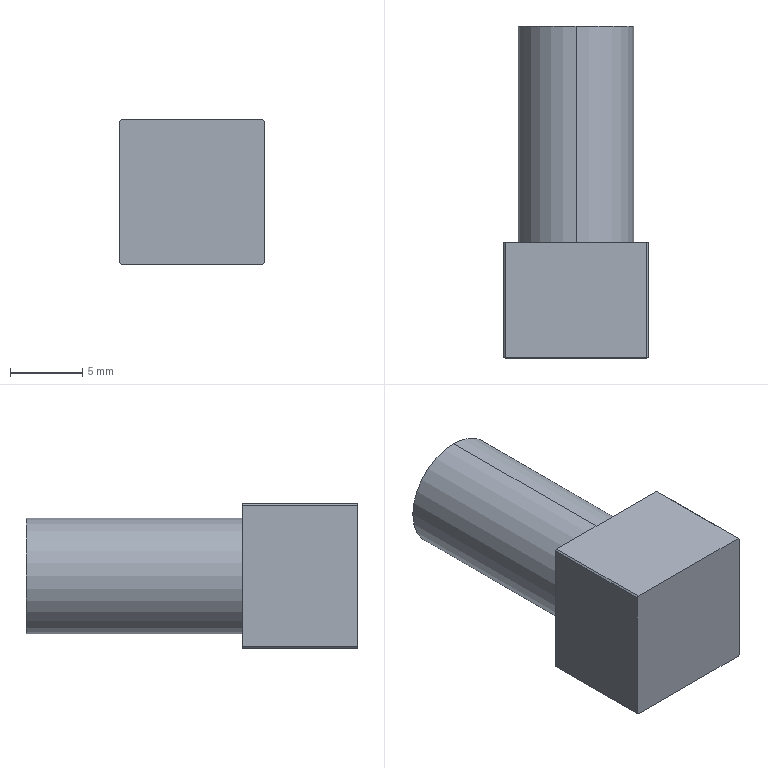Part | STEP file | 1 solid | 13 faces | box 10 x 23 x 10 mm | volume 1554 mm3 | plane 7 | cylinder 6 | commonest cylinder face diameters 14 x4 8 x2
STEP:
#1=CARTESIAN_POINT('',(0.,0.,0.));
#2=DIRECTION('',(0.,0.,1.));
#3=DIRECTION('',(1.,0.,0.));
#4=AXIS2_PLACEMENT_3D('',#1,#2,#3);
#5=CARTESIAN_POINT('',(0.,23.,-4.));
#6=VERTEX_POINT('',#5);
#7=CARTESIAN_POINT('',(0.,23.,4.));
#8=VERTEX_POINT('',#7);
#9=CARTESIAN_POINT('',(0.,23.,0.));
#10=DIRECTION('',(0.,-1.,0.));
#11=DIRECTION('',(0.,0.,-1.));
#12=AXIS2_PLACEMENT_3D('',#9,#10,#11);
#13=CIRCLE('',#12,4.);
#14=CARTESIAN_POINT('',(0.,0.,0.));
#15=DIRECTION('',(0.,-1.,0.));
#16=DIRECTION('',(0.,0.,-1.));
#17=AXIS2_PLACEMENT_3D('',#14,#15,#16);
#18=CYLINDRICAL_SURFACE('',#17,4.);
#19=CARTESIAN_POINT('',(0.,-23.));
#20=DIRECTION('',(1.,0.));
#21=VECTOR('',#20,1.);
#22=LINE('',#19,#21);
#23=(GEOMETRIC_REPRESENTATION_CONTEXT(2)PARAMETRIC_REPRESENTATION_CONTEXT()REPRESENTATION_CONTEXT('',''));
#24=DEFINITIONAL_REPRESENTATION('',(#22),#23);
#25=PCURVE('',#18,#24);
#26=CARTESIAN_POINT('',(4.,23.,0.));
#27=DIRECTION('',(0.,1.,0.));
#28=DIRECTION('',(0.,0.,1.));
#29=AXIS2_PLACEMENT_3D('',#26,#27,#28);
#30=PLANE('',#29);
#31=CARTESIAN_POINT('',(-4.,-4.));
#32=CARTESIAN_POINT('',(-4.,2.928));
#33=CARTESIAN_POINT('',(2.,-0.5359));
#34=CARTESIAN_POINT('',(8.,-4.));
#35=CARTESIAN_POINT('',(2.,-7.464));
#36=CARTESIAN_POINT('',(-4.,-10.928));
#37=CARTESIAN_POINT('',(-4.,-4.));
#38=(BOUNDED_CURVE()B_SPLINE_CURVE(2,(#31,#32,#33,#34,#35,#36,#37),.UNSPECIFIED.,.T.,.F.)B_SPLINE_CURVE_WITH_KNOTS((1,2,2,2,2,1),(-2.094,0.,2.094,4.189,6.283,8.378),.UNSPECIFIED.)CURVE()GEOMETRIC_REPRESENTATION_ITEM()RATIONAL_B_SPLINE_CURVE((1.,0.5,1.,0.5,1.,0.5,1.))REPRESENTATION_ITEM(''));
#39=(GEOMETRIC_REPRESENTATION_CONTEXT(2)PARAMETRIC_REPRESENTATION_CONTEXT()REPRESENTATION_CONTEXT('',''));
#40=DEFINITIONAL_REPRESENTATION('',(#38),#39);
#41=PCURVE('',#30,#40);
#42=SURFACE_CURVE('',#13,(#25,#41),.PCURVE_S1.);
#43=EDGE_CURVE('',#6,#8,#42,.T.);
#44=ORIENTED_EDGE('',*,*,#43,.T.);
#45=CARTESIAN_POINT('',(0.,8.,4.));
#46=VERTEX_POINT('',#45);
#47=CARTESIAN_POINT('',(0.,0.,4.));
#48=DIRECTION('',(0.,-1.,0.));
#49=VECTOR('',#48,1.);
#50=LINE('',#47,#49);
#51=CARTESIAN_POINT('',(3.142,0.));
#52=DIRECTION('',(0.,1.));
#53=VECTOR('',#52,1.);
#54=LINE('',#51,#53);
#55=(GEOMETRIC_REPRESENTATION_CONTEXT(2)PARAMETRIC_REPRESENTATION_CONTEXT()REPRESENTATION_CONTEXT('',''));
#56=DEFINITIONAL_REPRESENTATION('',(#54),#55);
#57=PCURVE('',#18,#56);
#58=CARTESIAN_POINT('',(0.,0.,0.));
#59=DIRECTION('',(0.,-1.,0.));
#60=DIRECTION('',(0.,0.,-1.));
#61=AXIS2_PLACEMENT_3D('',#58,#59,#60);
#62=CYLINDRICAL_SURFACE('',#61,4.);
#63=CARTESIAN_POINT('',(3.142,0.));
#64=DIRECTION('',(0.,1.));
#65=VECTOR('',#64,1.);
#66=LINE('',#63,#65);
#67=(GEOMETRIC_REPRESENTATION_CONTEXT(2)PARAMETRIC_REPRESENTATION_CONTEXT()REPRESENTATION_CONTEXT('',''));
#68=DEFINITIONAL_REPRESENTATION('',(#66),#67);
#69=PCURVE('',#62,#68);
#70=SURFACE_CURVE('',#50,(#57,#69),.PCURVE_S1.);
#71=EDGE_CURVE('',#8,#46,#70,.T.);
#72=ORIENTED_EDGE('',*,*,#71,.T.);
#73=CARTESIAN_POINT('',(0.,8.,-4.));
#74=VERTEX_POINT('',#73);
#75=CARTESIAN_POINT('',(0.,8.,0.));
#76=DIRECTION('',(0.,-1.,0.));
#77=DIRECTION('',(0.,0.,-1.));
#78=AXIS2_PLACEMENT_3D('',#75,#76,#77);
#79=CIRCLE('',#78,4.);
#80=CARTESIAN_POINT('',(0.,-8.));
#81=DIRECTION('',(1.,0.));
#82=VECTOR('',#81,1.);
#83=LINE('',#80,#82);
#84=(GEOMETRIC_REPRESENTATION_CONTEXT(2)PARAMETRIC_REPRESENTATION_CONTEXT()REPRESENTATION_CONTEXT('',''));
#85=DEFINITIONAL_REPRESENTATION('',(#83),#84);
#86=PCURVE('',#18,#85);
#87=CARTESIAN_POINT('',(7.,8.,0.));
#88=DIRECTION('',(0.,1.,0.));
#89=DIRECTION('',(0.,0.,1.));
#90=AXIS2_PLACEMENT_3D('',#87,#88,#89);
#91=PLANE('',#90);
#92=CARTESIAN_POINT('',(-4.,-7.));
#93=CARTESIAN_POINT('',(-4.,-0.0718));
#94=CARTESIAN_POINT('',(2.,-3.536));
#95=CARTESIAN_POINT('',(8.,-7.));
#96=CARTESIAN_POINT('',(2.,-10.464));
#97=CARTESIAN_POINT('',(-4.,-13.928));
#98=CARTESIAN_POINT('',(-4.,-7.));
#99=(BOUNDED_CURVE()B_SPLINE_CURVE(2,(#92,#93,#94,#95,#96,#97,#98),.UNSPECIFIED.,.T.,.F.)B_SPLINE_CURVE_WITH_KNOTS((1,2,2,2,2,1),(-2.094,0.,2.094,4.189,6.283,8.378),.UNSPECIFIED.)CURVE()GEOMETRIC_REPRESENTATION_ITEM()RATIONAL_B_SPLINE_CURVE((1.,0.5,1.,0.5,1.,0.5,1.))REPRESENTATION_ITEM(''));
#100=(GEOMETRIC_REPRESENTATION_CONTEXT(2)PARAMETRIC_REPRESENTATION_CONTEXT()REPRESENTATION_CONTEXT('',''));
#101=DEFINITIONAL_REPRESENTATION('',(#99),#100);
#102=PCURVE('',#91,#101);
#103=SURFACE_CURVE('',#79,(#86,#102),.PCURVE_S1.);
#104=EDGE_CURVE('',#74,#46,#103,.T.);
#105=ORIENTED_EDGE('',*,*,#104,.F.);
#106=CARTESIAN_POINT('',(0.,0.,-4.));
#107=DIRECTION('',(0.,-1.,0.));
#108=VECTOR('',#107,1.);
#109=LINE('',#106,#108);
#110=CARTESIAN_POINT('',(0.,0.));
#111=DIRECTION('',(0.,1.));
#112=VECTOR('',#111,1.);
#113=LINE('',#110,#112);
#114=(GEOMETRIC_REPRESENTATION_CONTEXT(2)PARAMETRIC_REPRESENTATION_CONTEXT()REPRESENTATION_CONTEXT('',''));
#115=DEFINITIONAL_REPRESENTATION('',(#113),#114);
#116=PCURVE('',#18,#115);
#117=CARTESIAN_POINT('',(6.283,0.));
#118=DIRECTION('',(0.,1.));
#119=VECTOR('',#118,1.);
#120=LINE('',#117,#119);
#121=(GEOMETRIC_REPRESENTATION_CONTEXT(2)PARAMETRIC_REPRESENTATION_CONTEXT()REPRESENTATION_CONTEXT('',''));
#122=DEFINITIONAL_REPRESENTATION('',(#120),#121);
#123=PCURVE('',#62,#122);
#124=SURFACE_CURVE('',#109,(#116,#123),.PCURVE_S1.);
#125=EDGE_CURVE('',#6,#74,#124,.T.);
#126=ORIENTED_EDGE('',*,*,#125,.F.);
#127=EDGE_LOOP('',(#44,#72,#105,#126));
#128=FACE_BOUND('',#127,.T.);
#129=ADVANCED_FACE('',(#128),#18,.T.);
#130=CARTESIAN_POINT('',(5.,0.,-4.899));
#131=VERTEX_POINT('',#130);
#132=CARTESIAN_POINT('',(5.,8.,-4.899));
#133=VERTEX_POINT('',#132);
#134=CARTESIAN_POINT('',(5.,0.,-4.899));
#135=DIRECTION('',(0.,1.,0.));
#136=VECTOR('',#135,1.);
#137=LINE('',#134,#136);
#138=CARTESIAN_POINT('',(0.,0.,0.));
#139=DIRECTION('',(0.,-1.,0.));
#140=DIRECTION('',(0.,0.,-1.));
#141=AXIS2_PLACEMENT_3D('',#138,#139,#140);
#142=CYLINDRICAL_SURFACE('',#141,7.);
#143=CARTESIAN_POINT('',(0.7956,0.));
#144=DIRECTION('',(0.,-1.));
#145=VECTOR('',#144,1.);
#146=LINE('',#143,#145);
#147=(GEOMETRIC_REPRESENTATION_CONTEXT(2)PARAMETRIC_REPRESENTATION_CONTEXT()REPRESENTATION_CONTEXT('',''));
#148=DEFINITIONAL_REPRESENTATION('',(#146),#147);
#149=PCURVE('',#142,#148);
#150=CARTESIAN_POINT('',(5.,23.,8.094));
#151=DIRECTION('',(-1.,0.,0.));
#152=DIRECTION('',(0.,0.,1.));
#153=AXIS2_PLACEMENT_3D('',#150,#151,#152);
#154=PLANE('',#153);
#155=CARTESIAN_POINT('',(-12.993,-23.));
#156=DIRECTION('',(0.,1.));
#157=VECTOR('',#156,1.);
#158=LINE('',#155,#157);
#159=(GEOMETRIC_REPRESENTATION_CONTEXT(2)PARAMETRIC_REPRESENTATION_CONTEXT()REPRESENTATION_CONTEXT('',''));
#160=DEFINITIONAL_REPRESENTATION('',(#158),#159);
#161=PCURVE('',#154,#160);
#162=SURFACE_CURVE('',#137,(#149,#161),.PCURVE_S1.);
#163=EDGE_CURVE('',#131,#133,#162,.T.);
#164=ORIENTED_EDGE('',*,*,#163,.F.);
#165=CARTESIAN_POINT('',(4.899,0.,-5.));
#166=VERTEX_POINT('',#165);
#167=CARTESIAN_POINT('',(0.,0.,0.));
#168=DIRECTION('',(0.,-1.,0.));
#169=DIRECTION('',(0.,0.,-1.));
#170=AXIS2_PLACEMENT_3D('',#167,#168,#169);
#171=CIRCLE('',#170,7.);
#172=CARTESIAN_POINT('',(0.,0.));
#173=DIRECTION('',(1.,0.));
#174=VECTOR('',#173,1.);
#175=LINE('',#172,#174);
#176=(GEOMETRIC_REPRESENTATION_CONTEXT(2)PARAMETRIC_REPRESENTATION_CONTEXT()REPRESENTATION_CONTEXT('',''));
#177=DEFINITIONAL_REPRESENTATION('',(#175),#176);
#178=PCURVE('',#142,#177);
#179=CARTESIAN_POINT('',(0.,0.,0.));
#180=DIRECTION('',(0.,-1.,0.));
#181=DIRECTION('',(0.,0.,-1.));
#182=AXIS2_PLACEMENT_3D('',#179,#180,#181);
#183=PLANE('',#182);
#184=CARTESIAN_POINT('',(0.,0.));
#185=DIRECTION('',(1.,0.));
#186=AXIS2_PLACEMENT_2D('',#184,#185);
#187=CIRCLE('',#186,7.);
#188=(GEOMETRIC_REPRESENTATION_CONTEXT(2)PARAMETRIC_REPRESENTATION_CONTEXT()REPRESENTATION_CONTEXT('',''));
#189=DEFINITIONAL_REPRESENTATION('',(#187),#188);
#190=PCURVE('',#183,#189);
#191=SURFACE_CURVE('',#171,(#178,#190),.PCURVE_S1.);
#192=EDGE_CURVE('',#166,#131,#191,.T.);
#193=ORIENTED_EDGE('',*,*,#192,.F.);
#194=CARTESIAN_POINT('',(4.899,8.,-5.));
#195=VERTEX_POINT('',#194);
#196=CARTESIAN_POINT('',(4.899,0.,-5.));
#197=DIRECTION('',(0.,-1.,0.));
#198=VECTOR('',#197,1.);
#199=LINE('',#196,#198);
#200=CARTESIAN_POINT('',(0.7752,0.));
#201=DIRECTION('',(0.,1.));
#202=VECTOR('',#201,1.);
#203=LINE('',#200,#202);
#204=(GEOMETRIC_REPRESENTATION_CONTEXT(2)PARAMETRIC_REPRESENTATION_CONTEXT()REPRESENTATION_CONTEXT('',''));
#205=DEFINITIONAL_REPRESENTATION('',(#203),#204);
#206=PCURVE('',#142,#205);
#207=CARTESIAN_POINT('',(-14.765,23.,-5.));
#208=DIRECTION('',(0.,0.,1.));
#209=DIRECTION('',(1.,0.,0.));
#210=AXIS2_PLACEMENT_3D('',#207,#208,#209);
#211=PLANE('',#210);
#212=CARTESIAN_POINT('',(19.664,-23.));
#213=DIRECTION('',(0.,-1.));
#214=VECTOR('',#213,1.);
#215=LINE('',#212,#214);
#216=(GEOMETRIC_REPRESENTATION_CONTEXT(2)PARAMETRIC_REPRESENTATION_CONTEXT()REPRESENTATION_CONTEXT('',''));
#217=DEFINITIONAL_REPRESENTATION('',(#215),#216);
#218=PCURVE('',#211,#217);
#219=SURFACE_CURVE('',#199,(#206,#218),.PCURVE_S1.);
#220=EDGE_CURVE('',#195,#166,#219,.T.);
#221=ORIENTED_EDGE('',*,*,#220,.F.);
#222=CARTESIAN_POINT('',(0.,8.,0.));
#223=DIRECTION('',(0.,-1.,0.));
#224=DIRECTION('',(0.,0.,-1.));
#225=AXIS2_PLACEMENT_3D('',#222,#223,#224);
#226=CIRCLE('',#225,7.);
#227=CARTESIAN_POINT('',(0.,-8.));
#228=DIRECTION('',(1.,0.));
#229=VECTOR('',#228,1.);
#230=LINE('',#227,#229);
#231=(GEOMETRIC_REPRESENTATION_CONTEXT(2)PARAMETRIC_REPRESENTATION_CONTEXT()REPRESENTATION_CONTEXT('',''));
#232=DEFINITIONAL_REPRESENTATION('',(#230),#231);
#233=PCURVE('',#142,#232);
#234=CARTESIAN_POINT('',(-7.,-7.));
#235=CARTESIAN_POINT('',(-7.,5.124));
#236=CARTESIAN_POINT('',(3.5,-0.9378));
#237=CARTESIAN_POINT('',(14.,-7.));
#238=CARTESIAN_POINT('',(3.5,-13.062));
#239=CARTESIAN_POINT('',(-7.,-19.124));
#240=CARTESIAN_POINT('',(-7.,-7.));
#241=(BOUNDED_CURVE()B_SPLINE_CURVE(2,(#234,#235,#236,#237,#238,#239,#240),.UNSPECIFIED.,.T.,.F.)B_SPLINE_CURVE_WITH_KNOTS((1,2,2,2,2,1),(-2.094,0.,2.094,4.189,6.283,8.378),.UNSPECIFIED.)CURVE()GEOMETRIC_REPRESENTATION_ITEM()RATIONAL_B_SPLINE_CURVE((1.,0.5,1.,0.5,1.,0.5,1.))REPRESENTATION_ITEM(''));
#242=(GEOMETRIC_REPRESENTATION_CONTEXT(2)PARAMETRIC_REPRESENTATION_CONTEXT()REPRESENTATION_CONTEXT('',''));
#243=DEFINITIONAL_REPRESENTATION('',(#241),#242);
#244=PCURVE('',#91,#243);
#245=SURFACE_CURVE('',#226,(#233,#244),.PCURVE_S1.);
#246=EDGE_CURVE('',#195,#133,#245,.T.);
#247=ORIENTED_EDGE('',*,*,#246,.T.);
#248=EDGE_LOOP('',(#164,#193,#221,#247));
#249=FACE_BOUND('',#248,.T.);
#250=ADVANCED_FACE('',(#249),#142,.T.);
#251=CARTESIAN_POINT('',(-5.,0.,4.899));
#252=VERTEX_POINT('',#251);
#253=CARTESIAN_POINT('',(-5.,8.,4.899));
#254=VERTEX_POINT('',#253);
#255=CARTESIAN_POINT('',(-5.,0.,4.899));
#256=DIRECTION('',(0.,1.,0.));
#257=VECTOR('',#256,1.);
#258=LINE('',#255,#257);
#259=CARTESIAN_POINT('',(0.,0.,0.));
#260=DIRECTION('',(0.,-1.,0.));
#261=DIRECTION('',(0.,0.,-1.));
#262=AXIS2_PLACEMENT_3D('',#259,#260,#261);
#263=CYLINDRICAL_SURFACE('',#262,7.);
#264=CARTESIAN_POINT('',(3.937,0.));
#265=DIRECTION('',(0.,-1.));
#266=VECTOR('',#265,1.);
#267=LINE('',#264,#266);
#268=(GEOMETRIC_REPRESENTATION_CONTEXT(2)PARAMETRIC_REPRESENTATION_CONTEXT()REPRESENTATION_CONTEXT('',''));
#269=DEFINITIONAL_REPRESENTATION('',(#267),#268);
#270=PCURVE('',#263,#269);
#271=CARTESIAN_POINT('',(-5.,23.,8.094));
#272=DIRECTION('',(1.,0.,0.));
#273=DIRECTION('',(0.,0.,-1.));
#274=AXIS2_PLACEMENT_3D('',#271,#272,#273);
#275=PLANE('',#274);
#276=CARTESIAN_POINT('',(3.195,-23.));
#277=DIRECTION('',(0.,1.));
#278=VECTOR('',#277,1.);
#279=LINE('',#276,#278);
#280=(GEOMETRIC_REPRESENTATION_CONTEXT(2)PARAMETRIC_REPRESENTATION_CONTEXT()REPRESENTATION_CONTEXT('',''));
#281=DEFINITIONAL_REPRESENTATION('',(#279),#280);
#282=PCURVE('',#275,#281);
#283=SURFACE_CURVE('',#258,(#270,#282),.PCURVE_S1.);
#284=EDGE_CURVE('',#252,#254,#283,.T.);
#285=ORIENTED_EDGE('',*,*,#284,.F.);
#286=CARTESIAN_POINT('',(-4.899,0.,5.));
#287=VERTEX_POINT('',#286);
#288=CARTESIAN_POINT('',(0.,0.,0.));
#289=DIRECTION('',(0.,-1.,0.));
#290=DIRECTION('',(0.,0.,-1.));
#291=AXIS2_PLACEMENT_3D('',#288,#289,#290);
#292=CIRCLE('',#291,7.);
#293=CARTESIAN_POINT('',(0.,0.));
#294=DIRECTION('',(1.,0.));
#295=VECTOR('',#294,1.);
#296=LINE('',#293,#295);
#297=(GEOMETRIC_REPRESENTATION_CONTEXT(2)PARAMETRIC_REPRESENTATION_CONTEXT()REPRESENTATION_CONTEXT('',''));
#298=DEFINITIONAL_REPRESENTATION('',(#296),#297);
#299=PCURVE('',#263,#298);
#300=CARTESIAN_POINT('',(0.,0.));
#301=DIRECTION('',(1.,0.));
#302=AXIS2_PLACEMENT_2D('',#300,#301);
#303=CIRCLE('',#302,7.);
#304=(GEOMETRIC_REPRESENTATION_CONTEXT(2)PARAMETRIC_REPRESENTATION_CONTEXT()REPRESENTATION_CONTEXT('',''));
#305=DEFINITIONAL_REPRESENTATION('',(#303),#304);
#306=PCURVE('',#183,#305);
#307=SURFACE_CURVE('',#292,(#299,#306),.PCURVE_S1.);
#308=EDGE_CURVE('',#287,#252,#307,.T.);
#309=ORIENTED_EDGE('',*,*,#308,.F.);
#310=CARTESIAN_POINT('',(-4.899,8.,5.));
#311=VERTEX_POINT('',#310);
#312=CARTESIAN_POINT('',(-4.899,0.,5.));
#313=DIRECTION('',(0.,-1.,0.));
#314=VECTOR('',#313,1.);
#315=LINE('',#312,#314);
#316=CARTESIAN_POINT('',(3.917,0.));
#317=DIRECTION('',(0.,1.));
#318=VECTOR('',#317,1.);
#319=LINE('',#316,#318);
#320=(GEOMETRIC_REPRESENTATION_CONTEXT(2)PARAMETRIC_REPRESENTATION_CONTEXT()REPRESENTATION_CONTEXT('',''));
#321=DEFINITIONAL_REPRESENTATION('',(#319),#320);
#322=PCURVE('',#263,#321);
#323=CARTESIAN_POINT('',(-11.017,23.,5.));
#324=DIRECTION('',(0.,0.,-1.));
#325=DIRECTION('',(-1.,0.,0.));
#326=AXIS2_PLACEMENT_3D('',#323,#324,#325);
#327=PLANE('',#326);
#328=CARTESIAN_POINT('',(-6.118,-23.));
#329=DIRECTION('',(0.,-1.));
#330=VECTOR('',#329,1.);
#331=LINE('',#328,#330);
#332=(GEOMETRIC_REPRESENTATION_CONTEXT(2)PARAMETRIC_REPRESENTATION_CONTEXT()REPRESENTATION_CONTEXT('',''));
#333=DEFINITIONAL_REPRESENTATION('',(#331),#332);
#334=PCURVE('',#327,#333);
#335=SURFACE_CURVE('',#315,(#322,#334),.PCURVE_S1.);
#336=EDGE_CURVE('',#311,#287,#335,.T.);
#337=ORIENTED_EDGE('',*,*,#336,.F.);
#338=CARTESIAN_POINT('',(0.,8.,0.));
#339=DIRECTION('',(0.,-1.,0.));
#340=DIRECTION('',(0.,0.,-1.));
#341=AXIS2_PLACEMENT_3D('',#338,#339,#340);
#342=CIRCLE('',#341,7.);
#343=CARTESIAN_POINT('',(0.,-8.));
#344=DIRECTION('',(1.,0.));
#345=VECTOR('',#344,1.);
#346=LINE('',#343,#345);
#347=(GEOMETRIC_REPRESENTATION_CONTEXT(2)PARAMETRIC_REPRESENTATION_CONTEXT()REPRESENTATION_CONTEXT('',''));
#348=DEFINITIONAL_REPRESENTATION('',(#346),#347);
#349=PCURVE('',#263,#348);
#350=CARTESIAN_POINT('',(-7.,-7.));
#351=CARTESIAN_POINT('',(-7.,5.124));
#352=CARTESIAN_POINT('',(3.5,-0.9378));
#353=CARTESIAN_POINT('',(14.,-7.));
#354=CARTESIAN_POINT('',(3.5,-13.062));
#355=CARTESIAN_POINT('',(-7.,-19.124));
#356=CARTESIAN_POINT('',(-7.,-7.));
#357=(BOUNDED_CURVE()B_SPLINE_CURVE(2,(#350,#351,#352,#353,#354,#355,#356),.UNSPECIFIED.,.T.,.F.)B_SPLINE_CURVE_WITH_KNOTS((1,2,2,2,2,1),(-2.094,0.,2.094,4.189,6.283,8.378),.UNSPECIFIED.)CURVE()GEOMETRIC_REPRESENTATION_ITEM()RATIONAL_B_SPLINE_CURVE((1.,0.5,1.,0.5,1.,0.5,1.))REPRESENTATION_ITEM(''));
#358=(GEOMETRIC_REPRESENTATION_CONTEXT(2)PARAMETRIC_REPRESENTATION_CONTEXT()REPRESENTATION_CONTEXT('',''));
#359=DEFINITIONAL_REPRESENTATION('',(#357),#358);
#360=PCURVE('',#91,#359);
#361=SURFACE_CURVE('',#342,(#349,#360),.PCURVE_S1.);
#362=EDGE_CURVE('',#311,#254,#361,.T.);
#363=ORIENTED_EDGE('',*,*,#362,.T.);
#364=EDGE_LOOP('',(#285,#309,#337,#363));
#365=FACE_BOUND('',#364,.T.);
#366=ADVANCED_FACE('',(#365),#263,.T.);
#367=CARTESIAN_POINT('',(5.,8.,4.899));
#368=VERTEX_POINT('',#367);
#369=CARTESIAN_POINT('',(5.,0.,4.899));
#370=VERTEX_POINT('',#369);
#371=CARTESIAN_POINT('',(5.,0.,4.899));
#372=DIRECTION('',(0.,-1.,0.));
#373=VECTOR('',#372,1.);
#374=LINE('',#371,#373);
#375=CARTESIAN_POINT('',(0.,0.,0.));
#376=DIRECTION('',(0.,-1.,0.));
#377=DIRECTION('',(0.,0.,-1.));
#378=AXIS2_PLACEMENT_3D('',#375,#376,#377);
#379=CYLINDRICAL_SURFACE('',#378,7.);
#380=CARTESIAN_POINT('',(2.346,0.));
#381=DIRECTION('',(0.,1.));
#382=VECTOR('',#381,1.);
#383=LINE('',#380,#382);
#384=(GEOMETRIC_REPRESENTATION_CONTEXT(2)PARAMETRIC_REPRESENTATION_CONTEXT()REPRESENTATION_CONTEXT('',''));
#385=DEFINITIONAL_REPRESENTATION('',(#383),#384);
#386=PCURVE('',#379,#385);
#387=CARTESIAN_POINT('',(-3.195,-23.));
#388=DIRECTION('',(0.,-1.));
#389=VECTOR('',#388,1.);
#390=LINE('',#387,#389);
#391=(GEOMETRIC_REPRESENTATION_CONTEXT(2)PARAMETRIC_REPRESENTATION_CONTEXT()REPRESENTATION_CONTEXT('',''));
#392=DEFINITIONAL_REPRESENTATION('',(#390),#391);
#393=PCURVE('',#154,#392);
#394=SURFACE_CURVE('',#374,(#386,#393),.PCURVE_S1.);
#395=EDGE_CURVE('',#368,#370,#394,.T.);
#396=ORIENTED_EDGE('',*,*,#395,.F.);
#397=CARTESIAN_POINT('',(4.899,8.,5.));
#398=VERTEX_POINT('',#397);
#399=CARTESIAN_POINT('',(0.,8.,0.));
#400=DIRECTION('',(0.,-1.,0.));
#401=DIRECTION('',(0.,0.,-1.));
#402=AXIS2_PLACEMENT_3D('',#399,#400,#401);
#403=CIRCLE('',#402,7.);
#404=CARTESIAN_POINT('',(0.,-8.));
#405=DIRECTION('',(1.,0.));
#406=VECTOR('',#405,1.);
#407=LINE('',#404,#406);
#408=(GEOMETRIC_REPRESENTATION_CONTEXT(2)PARAMETRIC_REPRESENTATION_CONTEXT()REPRESENTATION_CONTEXT('',''));
#409=DEFINITIONAL_REPRESENTATION('',(#407),#408);
#410=PCURVE('',#379,#409);
#411=CARTESIAN_POINT('',(-7.,-7.));
#412=CARTESIAN_POINT('',(-7.,5.124));
#413=CARTESIAN_POINT('',(3.5,-0.9378));
#414=CARTESIAN_POINT('',(14.,-7.));
#415=CARTESIAN_POINT('',(3.5,-13.062));
#416=CARTESIAN_POINT('',(-7.,-19.124));
#417=CARTESIAN_POINT('',(-7.,-7.));
#418=(BOUNDED_CURVE()B_SPLINE_CURVE(2,(#411,#412,#413,#414,#415,#416,#417),.UNSPECIFIED.,.T.,.F.)B_SPLINE_CURVE_WITH_KNOTS((1,2,2,2,2,1),(-2.094,0.,2.094,4.189,6.283,8.378),.UNSPECIFIED.)CURVE()GEOMETRIC_REPRESENTATION_ITEM()RATIONAL_B_SPLINE_CURVE((1.,0.5,1.,0.5,1.,0.5,1.))REPRESENTATION_ITEM(''));
#419=(GEOMETRIC_REPRESENTATION_CONTEXT(2)PARAMETRIC_REPRESENTATION_CONTEXT()REPRESENTATION_CONTEXT('',''));
#420=DEFINITIONAL_REPRESENTATION('',(#418),#419);
#421=PCURVE('',#91,#420);
#422=SURFACE_CURVE('',#403,(#410,#421),.PCURVE_S1.);
#423=EDGE_CURVE('',#368,#398,#422,.T.);
#424=ORIENTED_EDGE('',*,*,#423,.T.);
#425=CARTESIAN_POINT('',(4.899,0.,5.));
#426=VERTEX_POINT('',#425);
#427=CARTESIAN_POINT('',(4.899,0.,5.));
#428=DIRECTION('',(0.,1.,0.));
#429=VECTOR('',#428,1.);
#430=LINE('',#427,#429);
#431=CARTESIAN_POINT('',(2.366,0.));
#432=DIRECTION('',(0.,-1.));
#433=VECTOR('',#432,1.);
#434=LINE('',#431,#433);
#435=(GEOMETRIC_REPRESENTATION_CONTEXT(2)PARAMETRIC_REPRESENTATION_CONTEXT()REPRESENTATION_CONTEXT('',''));
#436=DEFINITIONAL_REPRESENTATION('',(#434),#435);
#437=PCURVE('',#379,#436);
#438=CARTESIAN_POINT('',(-15.916,-23.));
#439=DIRECTION('',(0.,1.));
#440=VECTOR('',#439,1.);
#441=LINE('',#438,#440);
#442=(GEOMETRIC_REPRESENTATION_CONTEXT(2)PARAMETRIC_REPRESENTATION_CONTEXT()REPRESENTATION_CONTEXT('',''));
#443=DEFINITIONAL_REPRESENTATION('',(#441),#442);
#444=PCURVE('',#327,#443);
#445=SURFACE_CURVE('',#430,(#437,#444),.PCURVE_S1.);
#446=EDGE_CURVE('',#426,#398,#445,.T.);
#447=ORIENTED_EDGE('',*,*,#446,.F.);
#448=CARTESIAN_POINT('',(0.,0.,0.));
#449=DIRECTION('',(0.,-1.,0.));
#450=DIRECTION('',(0.,0.,-1.));
#451=AXIS2_PLACEMENT_3D('',#448,#449,#450);
#452=CIRCLE('',#451,7.);
#453=CARTESIAN_POINT('',(0.,0.));
#454=DIRECTION('',(1.,0.));
#455=VECTOR('',#454,1.);
#456=LINE('',#453,#455);
#457=(GEOMETRIC_REPRESENTATION_CONTEXT(2)PARAMETRIC_REPRESENTATION_CONTEXT()REPRESENTATION_CONTEXT('',''));
#458=DEFINITIONAL_REPRESENTATION('',(#456),#457);
#459=PCURVE('',#379,#458);
#460=CARTESIAN_POINT('',(0.,0.));
#461=DIRECTION('',(1.,0.));
#462=AXIS2_PLACEMENT_2D('',#460,#461);
#463=CIRCLE('',#462,7.);
#464=(GEOMETRIC_REPRESENTATION_CONTEXT(2)PARAMETRIC_REPRESENTATION_CONTEXT()REPRESENTATION_CONTEXT('',''));
#465=DEFINITIONAL_REPRESENTATION('',(#463),#464);
#466=PCURVE('',#183,#465);
#467=SURFACE_CURVE('',#452,(#459,#466),.PCURVE_S1.);
#468=EDGE_CURVE('',#370,#426,#467,.T.);
#469=ORIENTED_EDGE('',*,*,#468,.F.);
#470=EDGE_LOOP('',(#396,#424,#447,#469));
#471=FACE_BOUND('',#470,.T.);
#472=ADVANCED_FACE('',(#471),#379,.T.);
#473=CARTESIAN_POINT('',(5.,0.,8.094));
#474=DIRECTION('',(0.,0.,-1.));
#475=VECTOR('',#474,1.);
#476=LINE('',#473,#475);
#477=CARTESIAN_POINT('',(-8.094,5.));
#478=DIRECTION('',(1.,0.));
#479=VECTOR('',#478,1.);
#480=LINE('',#477,#479);
#481=(GEOMETRIC_REPRESENTATION_CONTEXT(2)PARAMETRIC_REPRESENTATION_CONTEXT()REPRESENTATION_CONTEXT('',''));
#482=DEFINITIONAL_REPRESENTATION('',(#480),#481);
#483=PCURVE('',#183,#482);
#484=CARTESIAN_POINT('',(0.,-23.));
#485=DIRECTION('',(-1.,0.));
#486=VECTOR('',#485,1.);
#487=LINE('',#484,#486);
#488=(GEOMETRIC_REPRESENTATION_CONTEXT(2)PARAMETRIC_REPRESENTATION_CONTEXT()REPRESENTATION_CONTEXT('',''));
#489=DEFINITIONAL_REPRESENTATION('',(#487),#488);
#490=PCURVE('',#154,#489);
#491=SURFACE_CURVE('',#476,(#483,#490),.PCURVE_S1.);
#492=EDGE_CURVE('',#370,#131,#491,.T.);
#493=ORIENTED_EDGE('',*,*,#492,.F.);
#494=ORIENTED_EDGE('',*,*,#468,.T.);
#495=CARTESIAN_POINT('',(-11.017,0.,5.));
#496=DIRECTION('',(1.,0.,0.));
#497=VECTOR('',#496,1.);
#498=LINE('',#495,#497);
#499=CARTESIAN_POINT('',(-5.,-11.017));
#500=DIRECTION('',(0.,1.));
#501=VECTOR('',#500,1.);
#502=LINE('',#499,#501);
#503=(GEOMETRIC_REPRESENTATION_CONTEXT(2)PARAMETRIC_REPRESENTATION_CONTEXT()REPRESENTATION_CONTEXT('',''));
#504=DEFINITIONAL_REPRESENTATION('',(#502),#503);
#505=PCURVE('',#183,#504);
#506=CARTESIAN_POINT('',(0.,-23.));
#507=DIRECTION('',(-1.,0.));
#508=VECTOR('',#507,1.);
#509=LINE('',#506,#508);
#510=(GEOMETRIC_REPRESENTATION_CONTEXT(2)PARAMETRIC_REPRESENTATION_CONTEXT()REPRESENTATION_CONTEXT('',''));
#511=DEFINITIONAL_REPRESENTATION('',(#509),#510);
#512=PCURVE('',#327,#511);
#513=SURFACE_CURVE('',#498,(#505,#512),.PCURVE_S1.);
#514=EDGE_CURVE('',#287,#426,#513,.T.);
#515=ORIENTED_EDGE('',*,*,#514,.F.);
#516=ORIENTED_EDGE('',*,*,#308,.T.);
#517=CARTESIAN_POINT('',(-5.,0.,-4.899));
#518=VERTEX_POINT('',#517);
#519=CARTESIAN_POINT('',(-5.,0.,8.094));
#520=DIRECTION('',(0.,0.,1.));
#521=VECTOR('',#520,1.);
#522=LINE('',#519,#521);
#523=CARTESIAN_POINT('',(-8.094,-5.));
#524=DIRECTION('',(-1.,0.));
#525=VECTOR('',#524,1.);
#526=LINE('',#523,#525);
#527=(GEOMETRIC_REPRESENTATION_CONTEXT(2)PARAMETRIC_REPRESENTATION_CONTEXT()REPRESENTATION_CONTEXT('',''));
#528=DEFINITIONAL_REPRESENTATION('',(#526),#527);
#529=PCURVE('',#183,#528);
#530=CARTESIAN_POINT('',(0.,-23.));
#531=DIRECTION('',(-1.,0.));
#532=VECTOR('',#531,1.);
#533=LINE('',#530,#532);
#534=(GEOMETRIC_REPRESENTATION_CONTEXT(2)PARAMETRIC_REPRESENTATION_CONTEXT()REPRESENTATION_CONTEXT('',''));
#535=DEFINITIONAL_REPRESENTATION('',(#533),#534);
#536=PCURVE('',#275,#535);
#537=SURFACE_CURVE('',#522,(#529,#536),.PCURVE_S1.);
#538=EDGE_CURVE('',#518,#252,#537,.T.);
#539=ORIENTED_EDGE('',*,*,#538,.F.);
#540=CARTESIAN_POINT('',(-4.899,0.,-5.));
#541=VERTEX_POINT('',#540);
#542=CARTESIAN_POINT('',(0.,0.,0.));
#543=DIRECTION('',(0.,-1.,0.));
#544=DIRECTION('',(0.,0.,-1.));
#545=AXIS2_PLACEMENT_3D('',#542,#543,#544);
#546=CIRCLE('',#545,7.);
#547=CARTESIAN_POINT('',(0.,0.));
#548=DIRECTION('',(1.,0.));
#549=AXIS2_PLACEMENT_2D('',#547,#548);
#550=CIRCLE('',#549,7.);
#551=(GEOMETRIC_REPRESENTATION_CONTEXT(2)PARAMETRIC_REPRESENTATION_CONTEXT()REPRESENTATION_CONTEXT('',''));
#552=DEFINITIONAL_REPRESENTATION('',(#550),#551);
#553=PCURVE('',#183,#552);
#554=CARTESIAN_POINT('',(0.,0.,0.));
#555=DIRECTION('',(0.,-1.,0.));
#556=DIRECTION('',(0.,0.,-1.));
#557=AXIS2_PLACEMENT_3D('',#554,#555,#556);
#558=CYLINDRICAL_SURFACE('',#557,7.);
#559=CARTESIAN_POINT('',(0.,0.));
#560=DIRECTION('',(1.,0.));
#561=VECTOR('',#560,1.);
#562=LINE('',#559,#561);
#563=(GEOMETRIC_REPRESENTATION_CONTEXT(2)PARAMETRIC_REPRESENTATION_CONTEXT()REPRESENTATION_CONTEXT('',''));
#564=DEFINITIONAL_REPRESENTATION('',(#562),#563);
#565=PCURVE('',#558,#564);
#566=SURFACE_CURVE('',#546,(#553,#565),.PCURVE_S1.);
#567=EDGE_CURVE('',#518,#541,#566,.T.);
#568=ORIENTED_EDGE('',*,*,#567,.T.);
#569=CARTESIAN_POINT('',(-14.765,0.,-5.));
#570=DIRECTION('',(-1.,0.,0.));
#571=VECTOR('',#570,1.);
#572=LINE('',#569,#571);
#573=CARTESIAN_POINT('',(5.,-14.765));
#574=DIRECTION('',(0.,-1.));
#575=VECTOR('',#574,1.);
#576=LINE('',#573,#575);
#577=(GEOMETRIC_REPRESENTATION_CONTEXT(2)PARAMETRIC_REPRESENTATION_CONTEXT()REPRESENTATION_CONTEXT('',''));
#578=DEFINITIONAL_REPRESENTATION('',(#576),#577);
#579=PCURVE('',#183,#578);
#580=CARTESIAN_POINT('',(0.,-23.));
#581=DIRECTION('',(-1.,0.));
#582=VECTOR('',#581,1.);
#583=LINE('',#580,#582);
#584=(GEOMETRIC_REPRESENTATION_CONTEXT(2)PARAMETRIC_REPRESENTATION_CONTEXT()REPRESENTATION_CONTEXT('',''));
#585=DEFINITIONAL_REPRESENTATION('',(#583),#584);
#586=PCURVE('',#211,#585);
#587=SURFACE_CURVE('',#572,(#579,#586),.PCURVE_S1.);
#588=EDGE_CURVE('',#166,#541,#587,.T.);
#589=ORIENTED_EDGE('',*,*,#588,.F.);
#590=ORIENTED_EDGE('',*,*,#192,.T.);
#591=EDGE_LOOP('',(#493,#494,#515,#516,#539,#568,#589,#590));
#592=FACE_BOUND('',#591,.T.);
#593=ADVANCED_FACE('',(#592),#183,.T.);
#594=CARTESIAN_POINT('',(-5.,8.,-4.899));
#595=VERTEX_POINT('',#594);
#596=CARTESIAN_POINT('',(-5.,0.,-4.899));
#597=DIRECTION('',(0.,-1.,0.));
#598=VECTOR('',#597,1.);
#599=LINE('',#596,#598);
#600=CARTESIAN_POINT('',(5.488,0.));
#601=DIRECTION('',(0.,1.));
#602=VECTOR('',#601,1.);
#603=LINE('',#600,#602);
#604=(GEOMETRIC_REPRESENTATION_CONTEXT(2)PARAMETRIC_REPRESENTATION_CONTEXT()REPRESENTATION_CONTEXT('',''));
#605=DEFINITIONAL_REPRESENTATION('',(#603),#604);
#606=PCURVE('',#558,#605);
#607=CARTESIAN_POINT('',(12.993,-23.));
#608=DIRECTION('',(0.,-1.));
#609=VECTOR('',#608,1.);
#610=LINE('',#607,#609);
#611=(GEOMETRIC_REPRESENTATION_CONTEXT(2)PARAMETRIC_REPRESENTATION_CONTEXT()REPRESENTATION_CONTEXT('',''));
#612=DEFINITIONAL_REPRESENTATION('',(#610),#611);
#613=PCURVE('',#275,#612);
#614=SURFACE_CURVE('',#599,(#606,#613),.PCURVE_S1.);
#615=EDGE_CURVE('',#595,#518,#614,.T.);
#616=ORIENTED_EDGE('',*,*,#615,.F.);
#617=CARTESIAN_POINT('',(-4.899,8.,-5.));
#618=VERTEX_POINT('',#617);
#619=CARTESIAN_POINT('',(0.,8.,0.));
#620=DIRECTION('',(0.,-1.,0.));
#621=DIRECTION('',(0.,0.,-1.));
#622=AXIS2_PLACEMENT_3D('',#619,#620,#621);
#623=CIRCLE('',#622,7.);
#624=CARTESIAN_POINT('',(0.,-8.));
#625=DIRECTION('',(1.,0.));
#626=VECTOR('',#625,1.);
#627=LINE('',#624,#626);
#628=(GEOMETRIC_REPRESENTATION_CONTEXT(2)PARAMETRIC_REPRESENTATION_CONTEXT()REPRESENTATION_CONTEXT('',''));
#629=DEFINITIONAL_REPRESENTATION('',(#627),#628);
#630=PCURVE('',#558,#629);
#631=CARTESIAN_POINT('',(-7.,-7.));
#632=CARTESIAN_POINT('',(-7.,5.124));
#633=CARTESIAN_POINT('',(3.5,-0.9378));
#634=CARTESIAN_POINT('',(14.,-7.));
#635=CARTESIAN_POINT('',(3.5,-13.062));
#636=CARTESIAN_POINT('',(-7.,-19.124));
#637=CARTESIAN_POINT('',(-7.,-7.));
#638=(BOUNDED_CURVE()B_SPLINE_CURVE(2,(#631,#632,#633,#634,#635,#636,#637),.UNSPECIFIED.,.T.,.F.)B_SPLINE_CURVE_WITH_KNOTS((1,2,2,2,2,1),(-2.094,0.,2.094,4.189,6.283,8.378),.UNSPECIFIED.)CURVE()GEOMETRIC_REPRESENTATION_ITEM()RATIONAL_B_SPLINE_CURVE((1.,0.5,1.,0.5,1.,0.5,1.))REPRESENTATION_ITEM(''));
#639=(GEOMETRIC_REPRESENTATION_CONTEXT(2)PARAMETRIC_REPRESENTATION_CONTEXT()REPRESENTATION_CONTEXT('',''));
#640=DEFINITIONAL_REPRESENTATION('',(#638),#639);
#641=PCURVE('',#91,#640);
#642=SURFACE_CURVE('',#623,(#630,#641),.PCURVE_S1.);
#643=EDGE_CURVE('',#595,#618,#642,.T.);
#644=ORIENTED_EDGE('',*,*,#643,.T.);
#645=CARTESIAN_POINT('',(-4.899,0.,-5.));
#646=DIRECTION('',(0.,1.,0.));
#647=VECTOR('',#646,1.);
#648=LINE('',#645,#647);
#649=CARTESIAN_POINT('',(5.508,0.));
#650=DIRECTION('',(0.,-1.));
#651=VECTOR('',#650,1.);
#652=LINE('',#649,#651);
#653=(GEOMETRIC_REPRESENTATION_CONTEXT(2)PARAMETRIC_REPRESENTATION_CONTEXT()REPRESENTATION_CONTEXT('',''));
#654=DEFINITIONAL_REPRESENTATION('',(#652),#653);
#655=PCURVE('',#558,#654);
#656=CARTESIAN_POINT('',(9.866,-23.));
#657=DIRECTION('',(0.,1.));
#658=VECTOR('',#657,1.);
#659=LINE('',#656,#658);
#660=(GEOMETRIC_REPRESENTATION_CONTEXT(2)PARAMETRIC_REPRESENTATION_CONTEXT()REPRESENTATION_CONTEXT('',''));
#661=DEFINITIONAL_REPRESENTATION('',(#659),#660);
#662=PCURVE('',#211,#661);
#663=SURFACE_CURVE('',#648,(#655,#662),.PCURVE_S1.);
#664=EDGE_CURVE('',#541,#618,#663,.T.);
#665=ORIENTED_EDGE('',*,*,#664,.F.);
#666=ORIENTED_EDGE('',*,*,#567,.F.);
#667=EDGE_LOOP('',(#616,#644,#665,#666));
#668=FACE_BOUND('',#667,.T.);
#669=ADVANCED_FACE('',(#668),#558,.T.);
#670=CARTESIAN_POINT('',(5.,8.,0.));
#671=DIRECTION('',(0.,0.,1.));
#672=VECTOR('',#671,1.);
#673=LINE('',#670,#672);
#674=CARTESIAN_POINT('',(0.,-2.));
#675=DIRECTION('',(1.,0.));
#676=VECTOR('',#675,1.);
#677=LINE('',#674,#676);
#678=(GEOMETRIC_REPRESENTATION_CONTEXT(2)PARAMETRIC_REPRESENTATION_CONTEXT()REPRESENTATION_CONTEXT('',''));
#679=DEFINITIONAL_REPRESENTATION('',(#677),#678);
#680=PCURVE('',#91,#679);
#681=CARTESIAN_POINT('',(-8.094,-15.));
#682=DIRECTION('',(1.,0.));
#683=VECTOR('',#682,1.);
#684=LINE('',#681,#683);
#685=(GEOMETRIC_REPRESENTATION_CONTEXT(2)PARAMETRIC_REPRESENTATION_CONTEXT()REPRESENTATION_CONTEXT('',''));
#686=DEFINITIONAL_REPRESENTATION('',(#684),#685);
#687=PCURVE('',#154,#686);
#688=SURFACE_CURVE('',#673,(#680,#687),.PCURVE_S1.);
#689=EDGE_CURVE('',#133,#368,#688,.T.);
#690=ORIENTED_EDGE('',*,*,#689,.F.);
#691=ORIENTED_EDGE('',*,*,#246,.F.);
#692=CARTESIAN_POINT('',(7.,8.,-5.));
#693=DIRECTION('',(1.,0.,0.));
#694=VECTOR('',#693,1.);
#695=LINE('',#692,#694);
#696=CARTESIAN_POINT('',(-5.,0.));
#697=DIRECTION('',(0.,1.));
#698=VECTOR('',#697,1.);
#699=LINE('',#696,#698);
#700=(GEOMETRIC_REPRESENTATION_CONTEXT(2)PARAMETRIC_REPRESENTATION_CONTEXT()REPRESENTATION_CONTEXT('',''));
#701=DEFINITIONAL_REPRESENTATION('',(#699),#700);
#702=PCURVE('',#91,#701);
#703=CARTESIAN_POINT('',(21.765,-15.));
#704=DIRECTION('',(1.,0.));
#705=VECTOR('',#704,1.);
#706=LINE('',#703,#705);
#707=(GEOMETRIC_REPRESENTATION_CONTEXT(2)PARAMETRIC_REPRESENTATION_CONTEXT()REPRESENTATION_CONTEXT('',''));
#708=DEFINITIONAL_REPRESENTATION('',(#706),#707);
#709=PCURVE('',#211,#708);
#710=SURFACE_CURVE('',#695,(#702,#709),.PCURVE_S1.);
#711=EDGE_CURVE('',#618,#195,#710,.T.);
#712=ORIENTED_EDGE('',*,*,#711,.F.);
#713=ORIENTED_EDGE('',*,*,#643,.F.);
#714=CARTESIAN_POINT('',(-5.,8.,0.));
#715=DIRECTION('',(0.,0.,-1.));
#716=VECTOR('',#715,1.);
#717=LINE('',#714,#716);
#718=CARTESIAN_POINT('',(0.,-12.));
#719=DIRECTION('',(-1.,0.));
#720=VECTOR('',#719,1.);
#721=LINE('',#718,#720);
#722=(GEOMETRIC_REPRESENTATION_CONTEXT(2)PARAMETRIC_REPRESENTATION_CONTEXT()REPRESENTATION_CONTEXT('',''));
#723=DEFINITIONAL_REPRESENTATION('',(#721),#722);
#724=PCURVE('',#91,#723);
#725=CARTESIAN_POINT('',(8.094,-15.));
#726=DIRECTION('',(1.,0.));
#727=VECTOR('',#726,1.);
#728=LINE('',#725,#727);
#729=(GEOMETRIC_REPRESENTATION_CONTEXT(2)PARAMETRIC_REPRESENTATION_CONTEXT()REPRESENTATION_CONTEXT('',''));
#730=DEFINITIONAL_REPRESENTATION('',(#728),#729);
#731=PCURVE('',#275,#730);
#732=SURFACE_CURVE('',#717,(#724,#731),.PCURVE_S1.);
#733=EDGE_CURVE('',#254,#595,#732,.T.);
#734=ORIENTED_EDGE('',*,*,#733,.F.);
#735=ORIENTED_EDGE('',*,*,#362,.F.);
#736=CARTESIAN_POINT('',(7.,8.,5.));
#737=DIRECTION('',(-1.,0.,0.));
#738=VECTOR('',#737,1.);
#739=LINE('',#736,#738);
#740=CARTESIAN_POINT('',(5.,0.));
#741=DIRECTION('',(0.,-1.));
#742=VECTOR('',#741,1.);
#743=LINE('',#740,#742);
#744=(GEOMETRIC_REPRESENTATION_CONTEXT(2)PARAMETRIC_REPRESENTATION_CONTEXT()REPRESENTATION_CONTEXT('',''));
#745=DEFINITIONAL_REPRESENTATION('',(#743),#744);
#746=PCURVE('',#91,#745);
#747=CARTESIAN_POINT('',(-18.017,-15.));
#748=DIRECTION('',(1.,0.));
#749=VECTOR('',#748,1.);
#750=LINE('',#747,#749);
#751=(GEOMETRIC_REPRESENTATION_CONTEXT(2)PARAMETRIC_REPRESENTATION_CONTEXT()REPRESENTATION_CONTEXT('',''));
#752=DEFINITIONAL_REPRESENTATION('',(#750),#751);
#753=PCURVE('',#327,#752);
#754=SURFACE_CURVE('',#739,(#746,#753),.PCURVE_S1.);
#755=EDGE_CURVE('',#398,#311,#754,.T.);
#756=ORIENTED_EDGE('',*,*,#755,.F.);
#757=ORIENTED_EDGE('',*,*,#423,.F.);
#758=EDGE_LOOP('',(#690,#691,#712,#713,#734,#735,#756,#757));
#759=FACE_BOUND('',#758,.T.);
#760=ORIENTED_EDGE('',*,*,#104,.T.);
#761=CARTESIAN_POINT('',(0.,8.,0.));
#762=DIRECTION('',(0.,-1.,0.));
#763=DIRECTION('',(0.,0.,-1.));
#764=AXIS2_PLACEMENT_3D('',#761,#762,#763);
#765=CIRCLE('',#764,4.);
#766=CARTESIAN_POINT('',(-4.,-7.));
#767=CARTESIAN_POINT('',(-4.,-0.0718));
#768=CARTESIAN_POINT('',(2.,-3.536));
#769=CARTESIAN_POINT('',(8.,-7.));
#770=CARTESIAN_POINT('',(2.,-10.464));
#771=CARTESIAN_POINT('',(-4.,-13.928));
#772=CARTESIAN_POINT('',(-4.,-7.));
#773=(BOUNDED_CURVE()B_SPLINE_CURVE(2,(#766,#767,#768,#769,#770,#771,#772),.UNSPECIFIED.,.T.,.F.)B_SPLINE_CURVE_WITH_KNOTS((1,2,2,2,2,1),(-2.094,0.,2.094,4.189,6.283,8.378),.UNSPECIFIED.)CURVE()GEOMETRIC_REPRESENTATION_ITEM()RATIONAL_B_SPLINE_CURVE((1.,0.5,1.,0.5,1.,0.5,1.))REPRESENTATION_ITEM(''));
#774=(GEOMETRIC_REPRESENTATION_CONTEXT(2)PARAMETRIC_REPRESENTATION_CONTEXT()REPRESENTATION_CONTEXT('',''));
#775=DEFINITIONAL_REPRESENTATION('',(#773),#774);
#776=PCURVE('',#91,#775);
#777=CARTESIAN_POINT('',(0.,-8.));
#778=DIRECTION('',(1.,0.));
#779=VECTOR('',#778,1.);
#780=LINE('',#777,#779);
#781=(GEOMETRIC_REPRESENTATION_CONTEXT(2)PARAMETRIC_REPRESENTATION_CONTEXT()REPRESENTATION_CONTEXT('',''));
#782=DEFINITIONAL_REPRESENTATION('',(#780),#781);
#783=PCURVE('',#62,#782);
#784=SURFACE_CURVE('',#765,(#776,#783),.PCURVE_S1.);
#785=EDGE_CURVE('',#46,#74,#784,.T.);
#786=ORIENTED_EDGE('',*,*,#785,.T.);
#787=EDGE_LOOP('',(#760,#786));
#788=FACE_BOUND('',#787,.T.);
#789=ADVANCED_FACE('',(#759,#788),#91,.T.);
#790=ORIENTED_EDGE('',*,*,#71,.F.);
#791=CARTESIAN_POINT('',(0.,23.,0.));
#792=DIRECTION('',(0.,-1.,0.));
#793=DIRECTION('',(0.,0.,-1.));
#794=AXIS2_PLACEMENT_3D('',#791,#792,#793);
#795=CIRCLE('',#794,4.);
#796=CARTESIAN_POINT('',(0.,-23.));
#797=DIRECTION('',(1.,0.));
#798=VECTOR('',#797,1.);
#799=LINE('',#796,#798);
#800=(GEOMETRIC_REPRESENTATION_CONTEXT(2)PARAMETRIC_REPRESENTATION_CONTEXT()REPRESENTATION_CONTEXT('',''));
#801=DEFINITIONAL_REPRESENTATION('',(#799),#800);
#802=PCURVE('',#62,#801);
#803=CARTESIAN_POINT('',(-4.,-4.));
#804=CARTESIAN_POINT('',(-4.,2.928));
#805=CARTESIAN_POINT('',(2.,-0.5359));
#806=CARTESIAN_POINT('',(8.,-4.));
#807=CARTESIAN_POINT('',(2.,-7.464));
#808=CARTESIAN_POINT('',(-4.,-10.928));
#809=CARTESIAN_POINT('',(-4.,-4.));
#810=(BOUNDED_CURVE()B_SPLINE_CURVE(2,(#803,#804,#805,#806,#807,#808,#809),.UNSPECIFIED.,.T.,.F.)B_SPLINE_CURVE_WITH_KNOTS((1,2,2,2,2,1),(-2.094,0.,2.094,4.189,6.283,8.378),.UNSPECIFIED.)CURVE()GEOMETRIC_REPRESENTATION_ITEM()RATIONAL_B_SPLINE_CURVE((1.,0.5,1.,0.5,1.,0.5,1.))REPRESENTATION_ITEM(''));
#811=(GEOMETRIC_REPRESENTATION_CONTEXT(2)PARAMETRIC_REPRESENTATION_CONTEXT()REPRESENTATION_CONTEXT('',''));
#812=DEFINITIONAL_REPRESENTATION('',(#810),#811);
#813=PCURVE('',#30,#812);
#814=SURFACE_CURVE('',#795,(#802,#813),.PCURVE_S1.);
#815=EDGE_CURVE('',#8,#6,#814,.T.);
#816=ORIENTED_EDGE('',*,*,#815,.T.);
#817=ORIENTED_EDGE('',*,*,#125,.T.);
#818=ORIENTED_EDGE('',*,*,#785,.F.);
#819=EDGE_LOOP('',(#790,#816,#817,#818));
#820=FACE_BOUND('',#819,.T.);
#821=ADVANCED_FACE('',(#820),#62,.T.);
#822=ORIENTED_EDGE('',*,*,#43,.F.);
#823=ORIENTED_EDGE('',*,*,#815,.F.);
#824=EDGE_LOOP('',(#822,#823));
#825=FACE_BOUND('',#824,.T.);
#826=ADVANCED_FACE('',(#825),#30,.T.);
#827=ORIENTED_EDGE('',*,*,#664,.T.);
#828=ORIENTED_EDGE('',*,*,#711,.T.);
#829=ORIENTED_EDGE('',*,*,#220,.T.);
#830=ORIENTED_EDGE('',*,*,#588,.T.);
#831=EDGE_LOOP('',(#827,#828,#829,#830));
#832=FACE_BOUND('',#831,.T.);
#833=ADVANCED_FACE('',(#832),#211,.F.);
#834=ORIENTED_EDGE('',*,*,#446,.T.);
#835=ORIENTED_EDGE('',*,*,#755,.T.);
#836=ORIENTED_EDGE('',*,*,#336,.T.);
#837=ORIENTED_EDGE('',*,*,#514,.T.);
#838=EDGE_LOOP('',(#834,#835,#836,#837));
#839=FACE_BOUND('',#838,.T.);
#840=ADVANCED_FACE('',(#839),#327,.F.);
#841=ORIENTED_EDGE('',*,*,#284,.T.);
#842=ORIENTED_EDGE('',*,*,#733,.T.);
#843=ORIENTED_EDGE('',*,*,#615,.T.);
#844=ORIENTED_EDGE('',*,*,#538,.T.);
#845=EDGE_LOOP('',(#841,#842,#843,#844));
#846=FACE_BOUND('',#845,.T.);
#847=ADVANCED_FACE('',(#846),#275,.F.);
#848=ORIENTED_EDGE('',*,*,#163,.T.);
#849=ORIENTED_EDGE('',*,*,#689,.T.);
#850=ORIENTED_EDGE('',*,*,#395,.T.);
#851=ORIENTED_EDGE('',*,*,#492,.T.);
#852=EDGE_LOOP('',(#848,#849,#850,#851));
#853=FACE_BOUND('',#852,.T.);
#854=ADVANCED_FACE('',(#853),#154,.F.);
#855=CLOSED_SHELL('',(#129,#250,#366,#472,#593,#669,#789,#821,#826,#833,#840,#847,#854));
#856=MANIFOLD_SOLID_BREP('',#855);
#857=(LENGTH_UNIT()NAMED_UNIT(*)SI_UNIT(.MILLI.,.METRE.));
#858=UNCERTAINTY_MEASURE_WITH_UNIT(LENGTH_MEASURE(0.0000001),#857,'','');
#859=(NAMED_UNIT(*)PLANE_ANGLE_UNIT()SI_UNIT($,.RADIAN.));
#860=(NAMED_UNIT(*)SI_UNIT($,.STERADIAN.)SOLID_ANGLE_UNIT());
#861=(GEOMETRIC_REPRESENTATION_CONTEXT(3)GLOBAL_UNCERTAINTY_ASSIGNED_CONTEXT((#858))GLOBAL_UNIT_ASSIGNED_CONTEXT((#857,#859,#860))REPRESENTATION_CONTEXT('',''));
#862=ADVANCED_BREP_SHAPE_REPRESENTATION('',(#4,#856),#861);